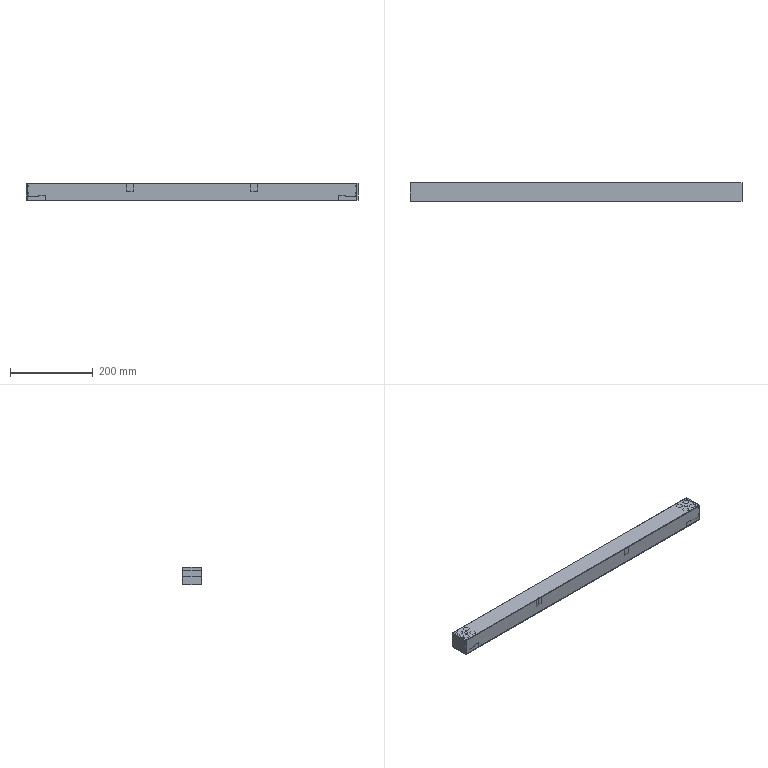CAM job | NX | 3-axis milling, drilling | part box 801.8 x 45 x 42 mm
Tools:
number,name,description,diameter,corner_radius,flute_length,length,flutes
1,D63,Milling Tool-5 Parameters,63.0,0.0,50.0,75.0,2
7,D6A45,Milling Tool-5 Parameters,6.0,0.0,3.0,3.0,2
12,7.8ZT,Drilling Tool,7.8,0.0,35.0,50.0,2
13,8.0JD,Milling Tool-5 Parameters,8.0,0.0,30.0,30.0,4
14,D14,Milling Tool-5 Parameters,14.0,0.0,50.0,75.0,2
10,D10,Milling Tool-5 Parameters,10.0,0.0,50.0,75.0,2
11,D10JING,Milling Tool-5 Parameters,10.0,0.0,50.0,75.0,2
8,8.5ZT,Drilling Tool,8.5,0.0,35.0,50.0,2
20,D12,Milling Tool-5 Parameters,12.0,0.0,50.0,75.0,2
21,D12JING,Milling Tool-5 Parameters,12.0,0.0,50.0,75.0,2
Operations:
program,operation,operation_type,tool,method,geometry_group,spindle_rpm,surface_speed,feed_per_tooth,feed_cut,feed_plunge,cut_length_mm,path_length_mm,cut_time_min,machine_time_min
22,FLOOR_WALL,VolumeBased25DMillingOperation,D63,METHOD,A,6500.0,1286.0,0.0962,1250.0,100.0,876.8,930.8,0.7014,0.7068
22,DRILLING_COPY_COPY_COPY_COPY,Operation,D14,METHOD,A,1200.0,52.0,0.0417,100.0,0.0,92.0,1126.228,0.92,1.023
22,ZLEVEL_PROFILE,ZLevelMilling,D10,METHOD,A,8000.0,251.0,0.2188,3500.0,100.0,840.395,1790.84,0.2401,0.3352
22,ZLEVEL_PROFILE_COPY,ZLevelMilling,D10JING,METHOD,A,8000.0,251.0,0.075,1200.0,100.0,122.262,1072.265,0.1019,0.1969
22,111,ZLevelMilling,D10JING,METHOD,A,8000.0,251.0,0.075,1200.0,100.0,238.747,857.309,0.199,0.2608
22,PLANAR_MILL,PlanarMilling,D6A45,METHOD,A,8000.0,150.0,0.0781,1250.0,100.0,2100.895,3654.902,1.681,1.836
11,FLOOR_WALL_COPY,VolumeBased25DMillingOperation,D63,METHOD,B,6500.0,1286.0,0.0962,1250.0,100.0,870.8,924.8,0.6966,0.702
11,ZLEVEL_PROFILE_COPY_2,ZLevelMilling,D12,METHOD,MCS_MILL_B,8000.0,251.0,0.2188,3500.0,100.0,5531.6,6626.693,1.581,1.69
11,FLOOR_WALL_1_1,VolumeBased25DMillingOperation,D10,METHOD,B,8000.0,251.0,0.1875,3000.0,1000.0,4939.621,5856.861,1.651,1.742
11,FLOOR_WALL_1_2,VolumeBased25DMillingOperation,D10,METHOD,B,8000.0,251.0,0.1875,3000.0,1000.0,460.0,1348.818,0.1747,0.2635
11,FLOOR_WALL_1_1_COPY,VolumeBased25DMillingOperation,D10,METHOD,B,8000.0,251.0,0.1875,3000.0,1000.0,459.419,1455.05,0.1573,0.2568
11,DRILLING_COPY_1,Operation,D6A45,METHOD,B,3000.0,56.0,0.0333,200.0,0.0,40.0,1065.773,0.2,0.3026
11,DRILLING_COPY_COPY_1,Operation,8.5ZT,METHOD,B,1500.0,42.0,0.0667,200.0,0.0,259.6,1479.851,1.298,1.42
11,DRILLING_COPY_COPY_COPY_1,Operation,7.8ZT,METHOD,B,1500.0,42.0,0.0667,200.0,0.0,75.687,982.379,0.3784,0.4691
11,DRILLING_COPY_COPY_COPY_COPY_1,Operation,8.0JD,METHOD,B,1000.0,25.0,0.0125,50.0,0.0,69.0,969.006,1.38,1.47
11,FLOOR_WALL_1_COPY,VolumeBased25DMillingOperation,D10JING,METHOD,B,8000.0,251.0,0.075,1200.0,1000.0,968.196,2319.707,0.8098,0.945
11,刀补11.,VolumeBased25DMillingOperation,D10JING,METHOD,B,8000.0,251.0,0.075,1200.0,1000.0,368.531,1510.035,0.3095,0.4237
11,刀补11_COPY,ZLevelMilling,D12JING,METHOD,B,8000.0,251.0,0.075,1200.0,100.0,132.201,318.272,0.1102,0.1288
11,ZLEVEL_PROFILE_COPY_1_COPY_COPY_COPY_COPY_2,ZLevelMilling,D6A45,METHOD,B,7000.0,131.0,0.0714,1000.0,1000.0,1518.689,1580.689,1.519,1.525
11,ZLEVEL_PROFILE_COPY_1_COPY_COPY_COPY_COPY_2_COPY,ZLevelMilling,D6A45,METHOD,B,7000.0,131.0,0.0714,1000.0,1000.0,448.156,2761.94,0.4482,0.6795
3,ZLEVEL_PROFILE_COPY_1,ZLevelMilling,D12JING,METHOD,B,6500.0,326.0,0.1538,2000.0,100.0,0.0,0.0,0.0,0.0,missing
3,ZLEVEL_PROFILE_COPY_1_1,ZLevelMilling,D12,METHOD,NONE,7500.0,235.0,0.2,3000.0,100.0,0.0,0.0,0.0,0.0,missing
3,刀补11,ZLevelMilling,D10JING,METHOD,A,8000.0,251.0,0.075,1200.0,100.0,253.575,1523.387,0.2113,0.3383